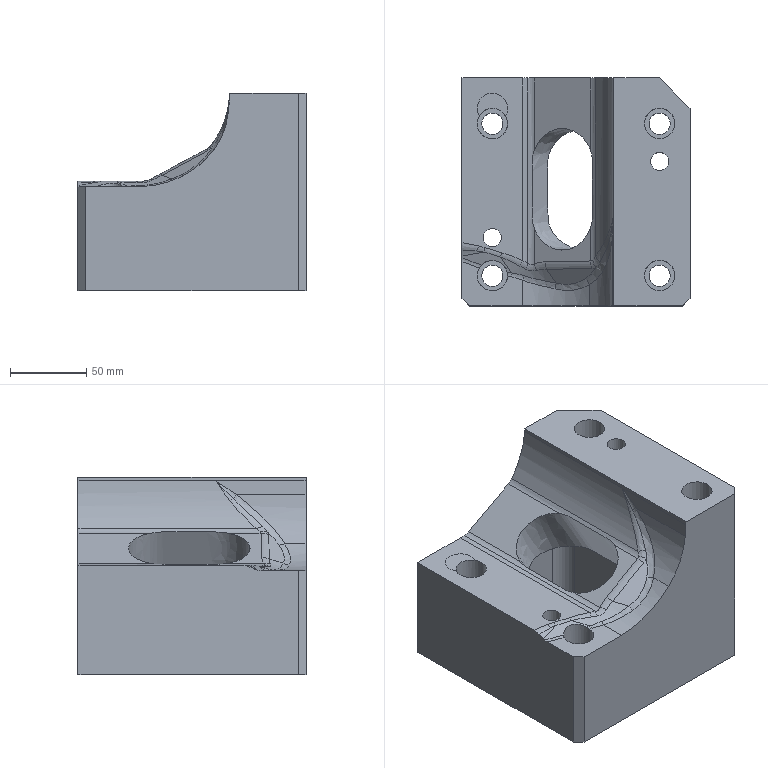Part | NX | features solid 2 | 1 solid | 69 faces | box 150 x 150 x 130 mm | volume 1538981 mm3 | plane 25 | spline 22 | cylinder 22 | commonest cylinder face diameters 20 x11 14 x4 12 x2 120 x2 16 x1 100 x1